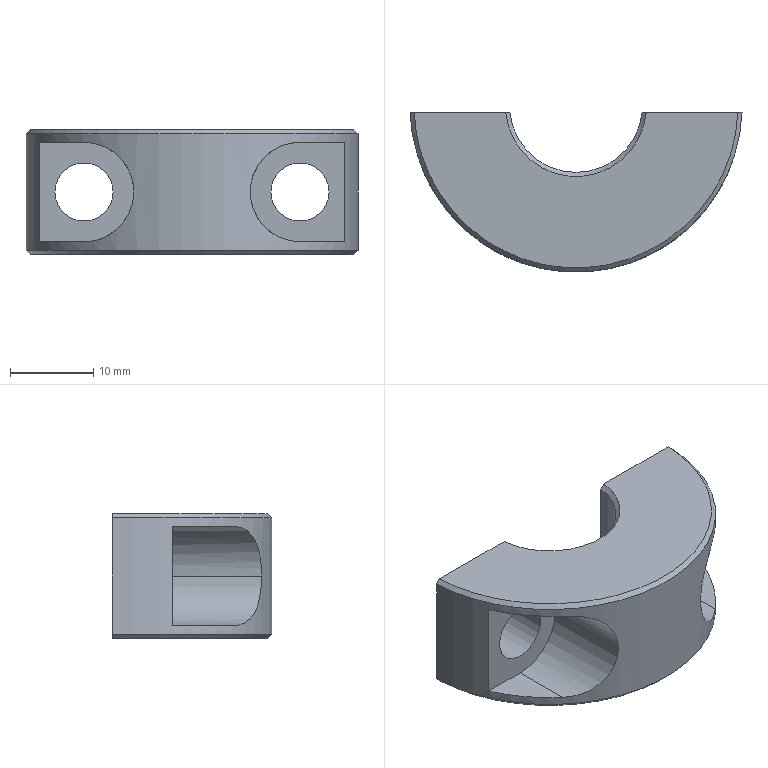Part | STEP file | 1_3 | 1 solid | 23 faces | box 39.972 x 19.25 x 15 mm | volume 5522 mm3 | plane 10 | cylinder 9 | cone 4 | commonest cylinder face diameters 7 x4 12 x3 16 x1 40 x1